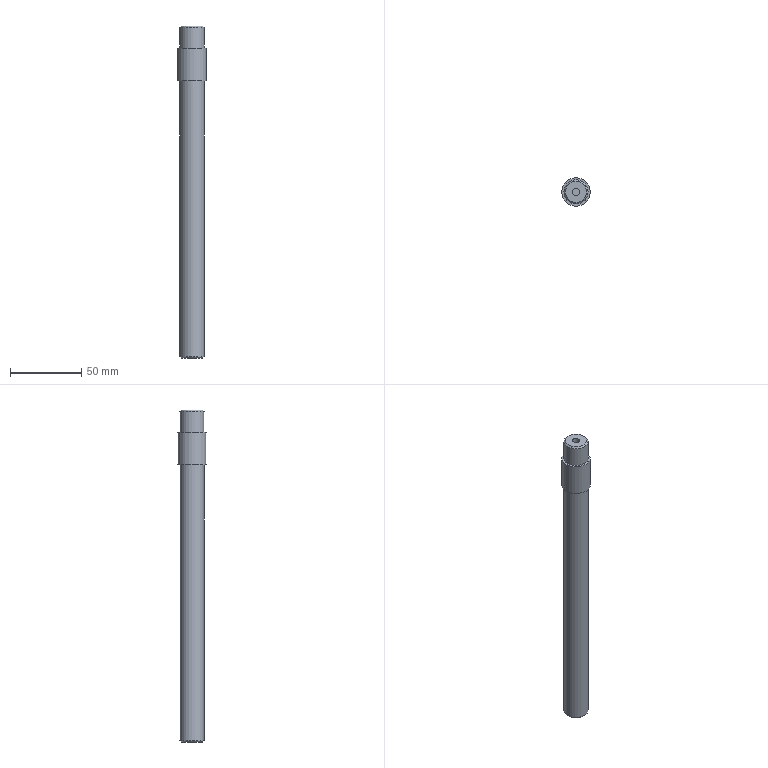Part | NX | features EXTRUDE 4, CHAMFER 2, DATUM_CSYS 1, LINKED_FACE 1, SKETCH 1, UNITE 1 | 1 solid | 13 faces | box 20 x 20 x 233 mm | volume 50412 mm3 | plane 6 | cylinder 5 | cone 2 | commonest cylinder face diameters 5 x2 17 x2 20 x1
STEP:
#1=CARTESIAN_POINT('',(8.5,0.,116.25));
#2=VERTEX_POINT('',#1);
#3=CARTESIAN_POINT('',(0.,0.,116.25));
#4=DIRECTION('',(0.,0.,1.));
#5=DIRECTION('',(1.,0.,0.));
#6=AXIS2_PLACEMENT_3D('',#3,#4,#5);
#7=CIRCLE('',#6,8.5);
#8=EDGE_CURVE('',#2,#2,#7,.F.);
#9=ORIENTED_EDGE('',*,*,#8,.T.);
#10=EDGE_LOOP('',(#9));
#11=FACE_BOUND('',#10,.T.);
#12=CARTESIAN_POINT('',(-8.5,0.,101.75));
#13=VERTEX_POINT('',#12);
#14=CARTESIAN_POINT('',(0.,0.,101.75));
#15=DIRECTION('',(0.,0.,1.));
#16=DIRECTION('',(-1.,0.,0.));
#17=AXIS2_PLACEMENT_3D('',#14,#15,#16);
#18=CIRCLE('',#17,8.5);
#19=EDGE_CURVE('',#13,#13,#18,.T.);
#20=ORIENTED_EDGE('',*,*,#19,.T.);
#21=EDGE_LOOP('',(#20));
#22=FACE_BOUND('',#21,.T.);
#23=CARTESIAN_POINT('',(0.,0.,101.75));
#24=DIRECTION('',(0.,0.,1.));
#25=DIRECTION('',(1.,0.,0.));
#26=AXIS2_PLACEMENT_3D('',#23,#24,#25);
#27=CYLINDRICAL_SURFACE('',#26,8.5);
#28=ADVANCED_FACE('',(#11,#22),#27,.T.);
#29=CARTESIAN_POINT('',(2.5,0.,117.25));
#30=VERTEX_POINT('',#29);
#31=CARTESIAN_POINT('',(0.,0.,117.25));
#32=DIRECTION('',(0.,0.,1.));
#33=DIRECTION('',(1.,0.,0.));
#34=AXIS2_PLACEMENT_3D('',#31,#32,#33);
#35=CIRCLE('',#34,2.5);
#36=EDGE_CURVE('',#30,#30,#35,.T.);
#37=ORIENTED_EDGE('',*,*,#36,.F.);
#38=EDGE_LOOP('',(#37));
#39=FACE_BOUND('',#38,.T.);
#40=CARTESIAN_POINT('',(7.5,0.,117.25));
#41=VERTEX_POINT('',#40);
#42=CARTESIAN_POINT('',(0.,0.,117.25));
#43=DIRECTION('',(0.,0.,1.));
#44=DIRECTION('',(1.,0.,0.));
#45=AXIS2_PLACEMENT_3D('',#42,#43,#44);
#46=CIRCLE('',#45,7.5);
#47=EDGE_CURVE('',#41,#41,#46,.T.);
#48=ORIENTED_EDGE('',*,*,#47,.T.);
#49=EDGE_LOOP('',(#48));
#50=FACE_BOUND('',#49,.T.);
#51=CARTESIAN_POINT('',(0.,0.,117.25));
#52=DIRECTION('',(0.,0.,1.));
#53=DIRECTION('',(1.,0.,0.));
#54=AXIS2_PLACEMENT_3D('',#51,#52,#53);
#55=PLANE('',#54);
#56=ADVANCED_FACE('',(#39,#50),#55,.T.);
#57=ORIENTED_EDGE('',*,*,#8,.F.);
#58=EDGE_LOOP('',(#57));
#59=FACE_BOUND('',#58,.T.);
#60=ORIENTED_EDGE('',*,*,#47,.F.);
#61=EDGE_LOOP('',(#60));
#62=FACE_BOUND('',#61,.T.);
#63=CARTESIAN_POINT('',(0.,0.,117.25));
#64=DIRECTION('',(0.,0.,-1.));
#65=DIRECTION('',(-1.,0.,0.));
#66=AXIS2_PLACEMENT_3D('',#63,#64,#65);
#67=CONICAL_SURFACE('',#66,7.5,0.7854);
#68=ADVANCED_FACE('',(#59,#62),#67,.T.);
#69=ORIENTED_EDGE('',*,*,#36,.T.);
#70=EDGE_LOOP('',(#69));
#71=FACE_BOUND('',#70,.T.);
#72=CARTESIAN_POINT('',(-2.5,0.,109.25));
#73=VERTEX_POINT('',#72);
#74=CARTESIAN_POINT('',(0.,0.,109.25));
#75=DIRECTION('',(0.,0.,1.));
#76=DIRECTION('',(-1.,0.,0.));
#77=AXIS2_PLACEMENT_3D('',#74,#75,#76);
#78=CIRCLE('',#77,2.5);
#79=EDGE_CURVE('',#73,#73,#78,.F.);
#80=ORIENTED_EDGE('',*,*,#79,.T.);
#81=EDGE_LOOP('',(#80));
#82=FACE_BOUND('',#81,.T.);
#83=CARTESIAN_POINT('',(0.,0.,109.25));
#84=DIRECTION('',(0.,0.,1.));
#85=DIRECTION('',(1.,0.,0.));
#86=AXIS2_PLACEMENT_3D('',#83,#84,#85);
#87=CYLINDRICAL_SURFACE('',#86,2.5);
#88=ADVANCED_FACE('',(#71,#82),#87,.F.);
#89=ORIENTED_EDGE('',*,*,#79,.F.);
#90=EDGE_LOOP('',(#89));
#91=FACE_BOUND('',#90,.T.);
#92=CARTESIAN_POINT('',(0.,0.,109.25));
#93=DIRECTION('',(0.,0.,1.));
#94=DIRECTION('',(1.,0.,0.));
#95=AXIS2_PLACEMENT_3D('',#92,#93,#94);
#96=PLANE('',#95);
#97=ADVANCED_FACE('',(#91),#96,.T.);
#98=CARTESIAN_POINT('',(10.,0.,101.75));
#99=VERTEX_POINT('',#98);
#100=CARTESIAN_POINT('',(0.,0.,101.75));
#101=DIRECTION('',(0.,0.,1.));
#102=DIRECTION('',(1.,0.,0.));
#103=AXIS2_PLACEMENT_3D('',#100,#101,#102);
#104=CIRCLE('',#103,10.);
#105=EDGE_CURVE('',#99,#99,#104,.T.);
#106=ORIENTED_EDGE('',*,*,#105,.T.);
#107=EDGE_LOOP('',(#106));
#108=FACE_BOUND('',#107,.T.);
#109=ORIENTED_EDGE('',*,*,#19,.F.);
#110=EDGE_LOOP('',(#109));
#111=FACE_BOUND('',#110,.T.);
#112=CARTESIAN_POINT('',(0.,0.,101.75));
#113=DIRECTION('',(0.,0.,1.));
#114=DIRECTION('',(1.,0.,0.));
#115=AXIS2_PLACEMENT_3D('',#112,#113,#114);
#116=PLANE('',#115);
#117=ADVANCED_FACE('',(#108,#111),#116,.T.);
#118=CARTESIAN_POINT('',(-10.,0.,78.75));
#119=VERTEX_POINT('',#118);
#120=CARTESIAN_POINT('',(0.,0.,78.75));
#121=DIRECTION('',(0.,0.,1.));
#122=DIRECTION('',(-1.,0.,0.));
#123=AXIS2_PLACEMENT_3D('',#120,#121,#122);
#124=CIRCLE('',#123,10.);
#125=EDGE_CURVE('',#119,#119,#124,.T.);
#126=ORIENTED_EDGE('',*,*,#125,.T.);
#127=EDGE_LOOP('',(#126));
#128=FACE_BOUND('',#127,.T.);
#129=ORIENTED_EDGE('',*,*,#105,.F.);
#130=EDGE_LOOP('',(#129));
#131=FACE_BOUND('',#130,.T.);
#132=CARTESIAN_POINT('',(0.,0.,101.75));
#133=DIRECTION('',(0.,0.,-1.));
#134=DIRECTION('',(-1.,0.,0.));
#135=AXIS2_PLACEMENT_3D('',#132,#133,#134);
#136=CYLINDRICAL_SURFACE('',#135,10.);
#137=ADVANCED_FACE('',(#128,#131),#136,.T.);
#138=ORIENTED_EDGE('',*,*,#125,.F.);
#139=EDGE_LOOP('',(#138));
#140=FACE_BOUND('',#139,.T.);
#141=CARTESIAN_POINT('',(-8.5,0.,78.75));
#142=VERTEX_POINT('',#141);
#143=CARTESIAN_POINT('',(0.,0.,78.75));
#144=DIRECTION('',(0.,0.,-1.));
#145=DIRECTION('',(-1.,0.,0.));
#146=AXIS2_PLACEMENT_3D('',#143,#144,#145);
#147=CIRCLE('',#146,8.5);
#148=EDGE_CURVE('',#142,#142,#147,.T.);
#149=ORIENTED_EDGE('',*,*,#148,.F.);
#150=EDGE_LOOP('',(#149));
#151=FACE_BOUND('',#150,.T.);
#152=CARTESIAN_POINT('',(0.,0.,78.75));
#153=DIRECTION('',(0.,0.,1.));
#154=DIRECTION('',(1.,0.,0.));
#155=AXIS2_PLACEMENT_3D('',#152,#153,#154);
#156=PLANE('',#155);
#157=ADVANCED_FACE('',(#140,#151),#156,.F.);
#158=CARTESIAN_POINT('',(8.5,0.,-114.75));
#159=VERTEX_POINT('',#158);
#160=CARTESIAN_POINT('',(0.,0.,-114.75));
#161=DIRECTION('',(0.,0.,1.));
#162=DIRECTION('',(1.,0.,0.));
#163=AXIS2_PLACEMENT_3D('',#160,#161,#162);
#164=CIRCLE('',#163,8.5);
#165=EDGE_CURVE('',#159,#159,#164,.T.);
#166=ORIENTED_EDGE('',*,*,#165,.T.);
#167=EDGE_LOOP('',(#166));
#168=FACE_BOUND('',#167,.T.);
#169=ORIENTED_EDGE('',*,*,#148,.T.);
#170=EDGE_LOOP('',(#169));
#171=FACE_BOUND('',#170,.T.);
#172=CARTESIAN_POINT('',(0.,0.,101.75));
#173=DIRECTION('',(0.,0.,-1.));
#174=DIRECTION('',(-1.,0.,0.));
#175=AXIS2_PLACEMENT_3D('',#172,#173,#174);
#176=CYLINDRICAL_SURFACE('',#175,8.5);
#177=ADVANCED_FACE('',(#168,#171),#176,.T.);
#178=CARTESIAN_POINT('',(-2.5,0.,-115.75));
#179=VERTEX_POINT('',#178);
#180=CARTESIAN_POINT('',(0.,0.,-115.75));
#181=DIRECTION('',(0.,0.,-1.));
#182=DIRECTION('',(-1.,0.,0.));
#183=AXIS2_PLACEMENT_3D('',#180,#181,#182);
#184=CIRCLE('',#183,2.5);
#185=EDGE_CURVE('',#179,#179,#184,.T.);
#186=ORIENTED_EDGE('',*,*,#185,.T.);
#187=EDGE_LOOP('',(#186));
#188=FACE_BOUND('',#187,.T.);
#189=CARTESIAN_POINT('',(2.5,0.,101.75));
#190=VERTEX_POINT('',#189);
#191=CARTESIAN_POINT('',(0.,0.,101.75));
#192=DIRECTION('',(0.,0.,-1.));
#193=DIRECTION('',(1.,0.,0.));
#194=AXIS2_PLACEMENT_3D('',#191,#192,#193);
#195=CIRCLE('',#194,2.5);
#196=EDGE_CURVE('',#190,#190,#195,.T.);
#197=ORIENTED_EDGE('',*,*,#196,.F.);
#198=EDGE_LOOP('',(#197));
#199=FACE_BOUND('',#198,.T.);
#200=CARTESIAN_POINT('',(0.,0.,101.75));
#201=DIRECTION('',(0.,0.,-1.));
#202=DIRECTION('',(-1.,0.,0.));
#203=AXIS2_PLACEMENT_3D('',#200,#201,#202);
#204=CYLINDRICAL_SURFACE('',#203,2.5);
#205=ADVANCED_FACE('',(#188,#199),#204,.F.);
#206=CARTESIAN_POINT('',(7.5,0.,-115.75));
#207=VERTEX_POINT('',#206);
#208=CARTESIAN_POINT('',(0.,0.,-115.75));
#209=DIRECTION('',(0.,0.,1.));
#210=DIRECTION('',(1.,0.,0.));
#211=AXIS2_PLACEMENT_3D('',#208,#209,#210);
#212=CIRCLE('',#211,7.5);
#213=EDGE_CURVE('',#207,#207,#212,.F.);
#214=ORIENTED_EDGE('',*,*,#213,.T.);
#215=EDGE_LOOP('',(#214));
#216=FACE_BOUND('',#215,.T.);
#217=ORIENTED_EDGE('',*,*,#185,.F.);
#218=EDGE_LOOP('',(#217));
#219=FACE_BOUND('',#218,.T.);
#220=CARTESIAN_POINT('',(0.,0.,-115.75));
#221=DIRECTION('',(0.,0.,1.));
#222=DIRECTION('',(1.,0.,0.));
#223=AXIS2_PLACEMENT_3D('',#220,#221,#222);
#224=PLANE('',#223);
#225=ADVANCED_FACE('',(#216,#219),#224,.F.);
#226=ORIENTED_EDGE('',*,*,#213,.F.);
#227=EDGE_LOOP('',(#226));
#228=FACE_BOUND('',#227,.T.);
#229=ORIENTED_EDGE('',*,*,#165,.F.);
#230=EDGE_LOOP('',(#229));
#231=FACE_BOUND('',#230,.T.);
#232=CARTESIAN_POINT('',(0.,0.,-114.75));
#233=DIRECTION('',(0.,0.,1.));
#234=DIRECTION('',(1.,0.,0.));
#235=AXIS2_PLACEMENT_3D('',#232,#233,#234);
#236=CONICAL_SURFACE('',#235,8.5,0.7854);
#237=ADVANCED_FACE('',(#228,#231),#236,.T.);
#238=ORIENTED_EDGE('',*,*,#196,.T.);
#239=EDGE_LOOP('',(#238));
#240=FACE_BOUND('',#239,.T.);
#241=CARTESIAN_POINT('',(0.,0.,101.75));
#242=DIRECTION('',(0.,0.,1.));
#243=DIRECTION('',(1.,0.,0.));
#244=AXIS2_PLACEMENT_3D('',#241,#242,#243);
#245=PLANE('',#244);
#246=ADVANCED_FACE('',(#240),#245,.F.);
#247=CLOSED_SHELL('',(#28,#56,#68,#88,#97,#117,#137,#157,#177,#205,#225,#237,#246));
#248=MANIFOLD_SOLID_BREP('',#247);
#249=(LENGTH_UNIT()NAMED_UNIT(*)SI_UNIT(.MILLI.,.METRE.));
#250=UNCERTAINTY_MEASURE_WITH_UNIT(LENGTH_MEASURE(0.00001),#249,'','');
#251=(NAMED_UNIT(*)PLANE_ANGLE_UNIT()SI_UNIT($,.RADIAN.));
#252=(NAMED_UNIT(*)SI_UNIT($,.STERADIAN.)SOLID_ANGLE_UNIT());
#253=(GEOMETRIC_REPRESENTATION_CONTEXT(3)GLOBAL_UNCERTAINTY_ASSIGNED_CONTEXT((#250))GLOBAL_UNIT_ASSIGNED_CONTEXT((#249,#251,#252))REPRESENTATION_CONTEXT('',''));
#254=ADVANCED_BREP_SHAPE_REPRESENTATION('',(#248),#253);